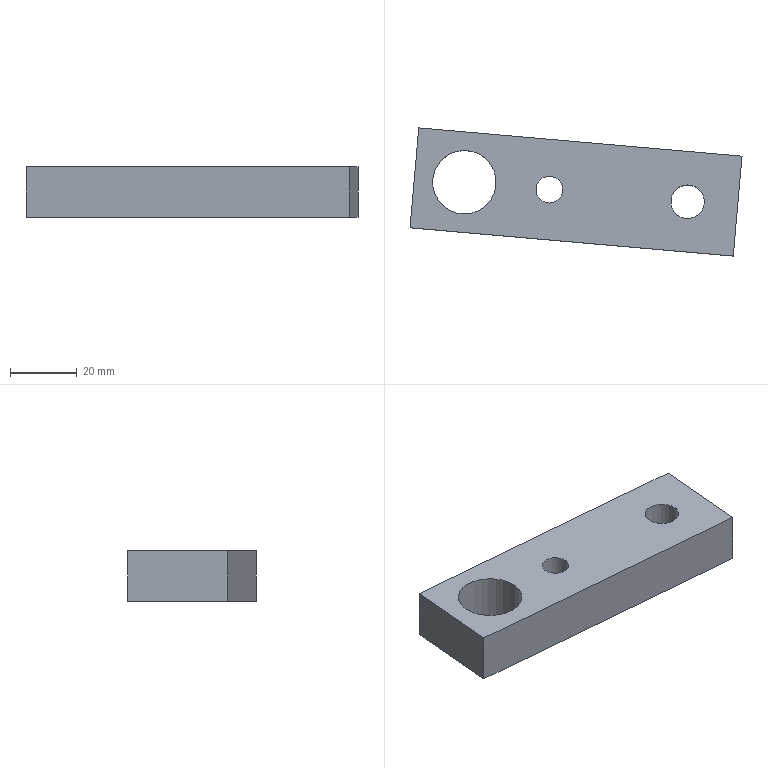Part | NX | features solid 2 | 1 solid | 9 faces | box 99.246 x 38.34 x 15 mm | volume 37465 mm3 | plane 6 | cylinder 3 | commonest cylinder face diameters 8 x1 10 x1 19 x1
STEP:
#1=CARTESIAN_POINT('',(-1457.005,422.796,-20.));
#2=VERTEX_POINT('',#1);
#3=CARTESIAN_POINT('',(-1459.619,392.91,-20.));
#4=VERTEX_POINT('',#3);
#5=CARTESIAN_POINT('',(-1457.005,422.796,-20.));
#6=DIRECTION('',(-0.08716,-0.9962,0.));
#7=VECTOR('',#6,1000.);
#8=LINE('',#5,#7);
#9=EDGE_CURVE('',#2,#4,#8,.T.);
#10=ORIENTED_EDGE('',*,*,#9,.F.);
#11=CARTESIAN_POINT('',(-1553.636,431.25,-20.));
#12=VERTEX_POINT('',#11);
#13=CARTESIAN_POINT('',(-1553.636,431.25,-20.));
#14=DIRECTION('',(0.9962,-0.08716,0.));
#15=VECTOR('',#14,1000.);
#16=LINE('',#13,#15);
#17=EDGE_CURVE('',#12,#2,#16,.T.);
#18=ORIENTED_EDGE('',*,*,#17,.F.);
#19=CARTESIAN_POINT('',(-1556.25,401.364,-20.));
#20=VERTEX_POINT('',#19);
#21=CARTESIAN_POINT('',(-1556.25,401.364,-20.));
#22=DIRECTION('',(0.08716,0.9962,0.));
#23=VECTOR('',#22,1000.);
#24=LINE('',#21,#23);
#25=EDGE_CURVE('',#20,#12,#24,.T.);
#26=ORIENTED_EDGE('',*,*,#25,.F.);
#27=CARTESIAN_POINT('',(-1459.619,392.91,-20.));
#28=DIRECTION('',(-0.9962,0.08716,0.));
#29=VECTOR('',#28,1000.);
#30=LINE('',#27,#29);
#31=EDGE_CURVE('',#4,#20,#30,.T.);
#32=ORIENTED_EDGE('',*,*,#31,.F.);
#33=EDGE_LOOP('',(#10,#18,#26,#32));
#34=FACE_BOUND('',#33,.T.);
#35=CARTESIAN_POINT('',(-1514.597,416.777,-20.));
#36=VERTEX_POINT('',#35);
#37=CARTESIAN_POINT('',(-1514.597,412.777,-20.));
#38=DIRECTION('',(0.,0.,-1.));
#39=DIRECTION('',(0.,1.,0.));
#40=AXIS2_PLACEMENT_3D('',#37,#38,#39);
#41=CIRCLE('',#40,4.);
#42=EDGE_CURVE('',#36,#36,#41,.T.);
#43=ORIENTED_EDGE('',*,*,#42,.T.);
#44=EDGE_LOOP('',(#43));
#45=FACE_BOUND('',#44,.T.);
#46=CARTESIAN_POINT('',(-1473.255,404.161,-20.));
#47=VERTEX_POINT('',#46);
#48=CARTESIAN_POINT('',(-1473.255,409.161,-20.));
#49=DIRECTION('',(0.,0.,-1.));
#50=DIRECTION('',(0.,-1.,0.));
#51=AXIS2_PLACEMENT_3D('',#48,#49,#50);
#52=CIRCLE('',#51,5.);
#53=EDGE_CURVE('',#47,#47,#52,.T.);
#54=ORIENTED_EDGE('',*,*,#53,.T.);
#55=EDGE_LOOP('',(#54));
#56=FACE_BOUND('',#55,.T.);
#57=CARTESIAN_POINT('',(-1540.,424.5,-20.));
#58=VERTEX_POINT('',#57);
#59=CARTESIAN_POINT('',(-1540.,415.,-20.));
#60=DIRECTION('',(0.,0.,-1.));
#61=DIRECTION('',(0.,1.,0.));
#62=AXIS2_PLACEMENT_3D('',#59,#60,#61);
#63=CIRCLE('',#62,9.5);
#64=EDGE_CURVE('',#58,#58,#63,.F.);
#65=ORIENTED_EDGE('',*,*,#64,.F.);
#66=EDGE_LOOP('',(#65));
#67=FACE_BOUND('',#66,.T.);
#68=CARTESIAN_POINT('',(-1459.619,392.91,-20.));
#69=DIRECTION('',(0.,0.,-1.));
#70=DIRECTION('',(0.,1.,0.));
#71=AXIS2_PLACEMENT_3D('',#68,#69,#70);
#72=PLANE('',#71);
#73=ADVANCED_FACE('',(#34,#45,#56,#67),#72,.F.);
#74=CARTESIAN_POINT('',(-1457.005,422.796,-35.));
#75=VERTEX_POINT('',#74);
#76=CARTESIAN_POINT('',(-1459.619,392.91,-35.));
#77=VERTEX_POINT('',#76);
#78=CARTESIAN_POINT('',(-1457.005,422.796,-35.));
#79=DIRECTION('',(-0.08716,-0.9962,0.));
#80=VECTOR('',#79,1000.);
#81=LINE('',#78,#80);
#82=EDGE_CURVE('',#75,#77,#81,.T.);
#83=ORIENTED_EDGE('',*,*,#82,.T.);
#84=CARTESIAN_POINT('',(-1556.25,401.364,-35.));
#85=VERTEX_POINT('',#84);
#86=CARTESIAN_POINT('',(-1459.619,392.91,-35.));
#87=DIRECTION('',(-0.9962,0.08716,0.));
#88=VECTOR('',#87,1000.);
#89=LINE('',#86,#88);
#90=EDGE_CURVE('',#77,#85,#89,.T.);
#91=ORIENTED_EDGE('',*,*,#90,.T.);
#92=CARTESIAN_POINT('',(-1553.636,431.25,-35.));
#93=VERTEX_POINT('',#92);
#94=CARTESIAN_POINT('',(-1556.25,401.364,-35.));
#95=DIRECTION('',(0.08716,0.9962,0.));
#96=VECTOR('',#95,1000.);
#97=LINE('',#94,#96);
#98=EDGE_CURVE('',#85,#93,#97,.T.);
#99=ORIENTED_EDGE('',*,*,#98,.T.);
#100=CARTESIAN_POINT('',(-1553.636,431.25,-35.));
#101=DIRECTION('',(0.9962,-0.08716,0.));
#102=VECTOR('',#101,1000.);
#103=LINE('',#100,#102);
#104=EDGE_CURVE('',#93,#75,#103,.T.);
#105=ORIENTED_EDGE('',*,*,#104,.T.);
#106=EDGE_LOOP('',(#83,#91,#99,#105));
#107=FACE_BOUND('',#106,.T.);
#108=CARTESIAN_POINT('',(-1514.597,416.777,-35.));
#109=VERTEX_POINT('',#108);
#110=CARTESIAN_POINT('',(-1514.597,412.777,-35.));
#111=DIRECTION('',(0.,0.,-1.));
#112=DIRECTION('',(0.,1.,0.));
#113=AXIS2_PLACEMENT_3D('',#110,#111,#112);
#114=CIRCLE('',#113,4.);
#115=EDGE_CURVE('',#109,#109,#114,.T.);
#116=ORIENTED_EDGE('',*,*,#115,.F.);
#117=EDGE_LOOP('',(#116));
#118=FACE_BOUND('',#117,.T.);
#119=CARTESIAN_POINT('',(-1473.255,404.161,-35.));
#120=VERTEX_POINT('',#119);
#121=CARTESIAN_POINT('',(-1473.255,409.161,-35.));
#122=DIRECTION('',(0.,0.,-1.));
#123=DIRECTION('',(0.,-1.,0.));
#124=AXIS2_PLACEMENT_3D('',#121,#122,#123);
#125=CIRCLE('',#124,5.);
#126=EDGE_CURVE('',#120,#120,#125,.T.);
#127=ORIENTED_EDGE('',*,*,#126,.F.);
#128=EDGE_LOOP('',(#127));
#129=FACE_BOUND('',#128,.T.);
#130=CARTESIAN_POINT('',(-1540.,424.5,-35.));
#131=VERTEX_POINT('',#130);
#132=CARTESIAN_POINT('',(-1540.,415.,-35.));
#133=DIRECTION('',(0.,0.,1.));
#134=DIRECTION('',(0.,1.,0.));
#135=AXIS2_PLACEMENT_3D('',#132,#133,#134);
#136=CIRCLE('',#135,9.5);
#137=EDGE_CURVE('',#131,#131,#136,.T.);
#138=ORIENTED_EDGE('',*,*,#137,.T.);
#139=EDGE_LOOP('',(#138));
#140=FACE_BOUND('',#139,.T.);
#141=CARTESIAN_POINT('',(-1459.619,392.91,-35.));
#142=DIRECTION('',(0.,0.,-1.));
#143=DIRECTION('',(0.,1.,0.));
#144=AXIS2_PLACEMENT_3D('',#141,#142,#143);
#145=PLANE('',#144);
#146=ADVANCED_FACE('',(#107,#118,#129,#140),#145,.T.);
#147=ORIENTED_EDGE('',*,*,#82,.F.);
#148=CARTESIAN_POINT('',(-1457.005,422.796,-20.));
#149=DIRECTION('',(0.,0.,-1.));
#150=VECTOR('',#149,1000.);
#151=LINE('',#148,#150);
#152=EDGE_CURVE('',#2,#75,#151,.T.);
#153=ORIENTED_EDGE('',*,*,#152,.F.);
#154=ORIENTED_EDGE('',*,*,#9,.T.);
#155=CARTESIAN_POINT('',(-1459.619,392.91,-20.));
#156=DIRECTION('',(0.,0.,-1.));
#157=VECTOR('',#156,1000.);
#158=LINE('',#155,#157);
#159=EDGE_CURVE('',#4,#77,#158,.T.);
#160=ORIENTED_EDGE('',*,*,#159,.T.);
#161=EDGE_LOOP('',(#147,#153,#154,#160));
#162=FACE_BOUND('',#161,.T.);
#163=CARTESIAN_POINT('',(-1457.005,422.796,-20.));
#164=DIRECTION('',(0.9962,-0.08716,0.));
#165=DIRECTION('',(0.08716,0.9962,0.));
#166=AXIS2_PLACEMENT_3D('',#163,#164,#165);
#167=PLANE('',#166);
#168=ADVANCED_FACE('',(#162),#167,.T.);
#169=ORIENTED_EDGE('',*,*,#90,.F.);
#170=ORIENTED_EDGE('',*,*,#159,.F.);
#171=ORIENTED_EDGE('',*,*,#31,.T.);
#172=CARTESIAN_POINT('',(-1556.25,401.364,-20.));
#173=DIRECTION('',(0.,0.,-1.));
#174=VECTOR('',#173,1000.);
#175=LINE('',#172,#174);
#176=EDGE_CURVE('',#20,#85,#175,.T.);
#177=ORIENTED_EDGE('',*,*,#176,.T.);
#178=EDGE_LOOP('',(#169,#170,#171,#177));
#179=FACE_BOUND('',#178,.T.);
#180=CARTESIAN_POINT('',(-1459.619,392.91,-20.));
#181=DIRECTION('',(-0.08716,-0.9962,0.));
#182=DIRECTION('',(0.9962,-0.08716,0.));
#183=AXIS2_PLACEMENT_3D('',#180,#181,#182);
#184=PLANE('',#183);
#185=ADVANCED_FACE('',(#179),#184,.T.);
#186=ORIENTED_EDGE('',*,*,#98,.F.);
#187=ORIENTED_EDGE('',*,*,#176,.F.);
#188=ORIENTED_EDGE('',*,*,#25,.T.);
#189=CARTESIAN_POINT('',(-1553.636,431.25,-20.));
#190=DIRECTION('',(0.,0.,-1.));
#191=VECTOR('',#190,1000.);
#192=LINE('',#189,#191);
#193=EDGE_CURVE('',#12,#93,#192,.T.);
#194=ORIENTED_EDGE('',*,*,#193,.T.);
#195=EDGE_LOOP('',(#186,#187,#188,#194));
#196=FACE_BOUND('',#195,.T.);
#197=CARTESIAN_POINT('',(-1556.25,401.364,-20.));
#198=DIRECTION('',(-0.9962,0.08716,0.));
#199=DIRECTION('',(-0.08716,-0.9962,0.));
#200=AXIS2_PLACEMENT_3D('',#197,#198,#199);
#201=PLANE('',#200);
#202=ADVANCED_FACE('',(#196),#201,.T.);
#203=ORIENTED_EDGE('',*,*,#104,.F.);
#204=ORIENTED_EDGE('',*,*,#193,.F.);
#205=ORIENTED_EDGE('',*,*,#17,.T.);
#206=ORIENTED_EDGE('',*,*,#152,.T.);
#207=EDGE_LOOP('',(#203,#204,#205,#206));
#208=FACE_BOUND('',#207,.T.);
#209=CARTESIAN_POINT('',(-1553.636,431.25,-20.));
#210=DIRECTION('',(0.08716,0.9962,0.));
#211=DIRECTION('',(-0.9962,0.08716,0.));
#212=AXIS2_PLACEMENT_3D('',#209,#210,#211);
#213=PLANE('',#212);
#214=ADVANCED_FACE('',(#208),#213,.T.);
#215=ORIENTED_EDGE('',*,*,#115,.T.);
#216=EDGE_LOOP('',(#215));
#217=FACE_BOUND('',#216,.T.);
#218=ORIENTED_EDGE('',*,*,#42,.F.);
#219=EDGE_LOOP('',(#218));
#220=FACE_BOUND('',#219,.T.);
#221=CARTESIAN_POINT('',(-1514.597,412.777,-20.));
#222=DIRECTION('',(0.,0.,-1.));
#223=DIRECTION('',(0.,1.,0.));
#224=AXIS2_PLACEMENT_3D('',#221,#222,#223);
#225=CYLINDRICAL_SURFACE('',#224,4.);
#226=ADVANCED_FACE('',(#217,#220),#225,.F.);
#227=ORIENTED_EDGE('',*,*,#126,.T.);
#228=EDGE_LOOP('',(#227));
#229=FACE_BOUND('',#228,.T.);
#230=ORIENTED_EDGE('',*,*,#53,.F.);
#231=EDGE_LOOP('',(#230));
#232=FACE_BOUND('',#231,.T.);
#233=CARTESIAN_POINT('',(-1473.255,409.161,-65.004));
#234=DIRECTION('',(0.,0.,-1.));
#235=DIRECTION('',(0.,1.,0.));
#236=AXIS2_PLACEMENT_3D('',#233,#234,#235);
#237=CYLINDRICAL_SURFACE('',#236,5.);
#238=ADVANCED_FACE('',(#229,#232),#237,.F.);
#239=ORIENTED_EDGE('',*,*,#137,.F.);
#240=EDGE_LOOP('',(#239));
#241=FACE_BOUND('',#240,.T.);
#242=ORIENTED_EDGE('',*,*,#64,.T.);
#243=EDGE_LOOP('',(#242));
#244=FACE_BOUND('',#243,.T.);
#245=CARTESIAN_POINT('',(-1540.,415.,65.));
#246=DIRECTION('',(0.,0.,-1.));
#247=DIRECTION('',(-1.,0.,0.));
#248=AXIS2_PLACEMENT_3D('',#245,#246,#247);
#249=CYLINDRICAL_SURFACE('',#248,9.5);
#250=ADVANCED_FACE('',(#241,#244),#249,.F.);
#251=CLOSED_SHELL('',(#73,#146,#168,#185,#202,#214,#226,#238,#250));
#252=MANIFOLD_SOLID_BREP('',#251);
#253=(LENGTH_UNIT()NAMED_UNIT(*)SI_UNIT(.MILLI.,.METRE.));
#254=UNCERTAINTY_MEASURE_WITH_UNIT(LENGTH_MEASURE(0.00001),#253,'','');
#255=(NAMED_UNIT(*)PLANE_ANGLE_UNIT()SI_UNIT($,.RADIAN.));
#256=(NAMED_UNIT(*)SI_UNIT($,.STERADIAN.)SOLID_ANGLE_UNIT());
#257=(GEOMETRIC_REPRESENTATION_CONTEXT(3)GLOBAL_UNCERTAINTY_ASSIGNED_CONTEXT((#254))GLOBAL_UNIT_ASSIGNED_CONTEXT((#253,#255,#256))REPRESENTATION_CONTEXT('',''));
#258=ADVANCED_BREP_SHAPE_REPRESENTATION('',(#252),#257);